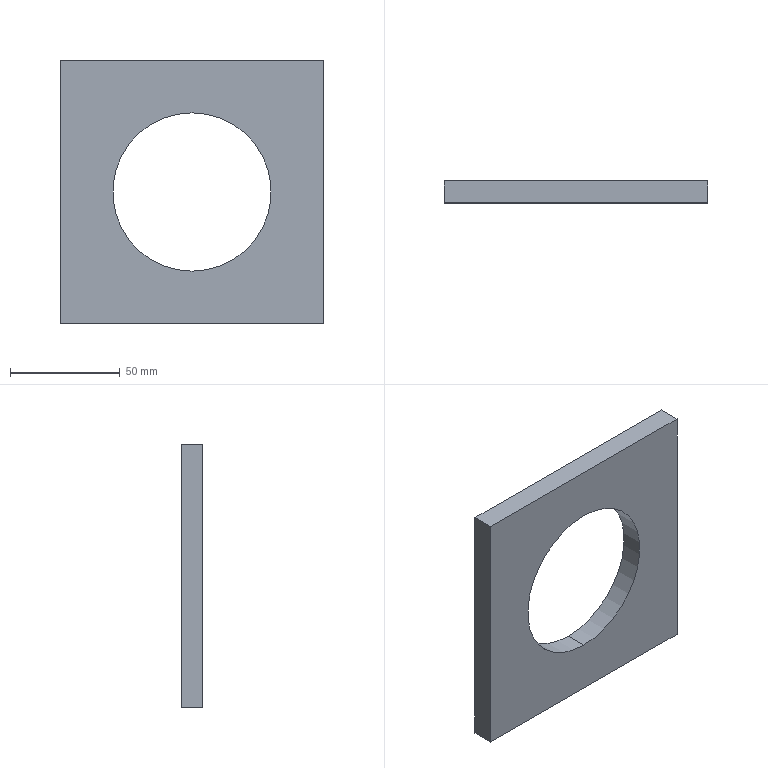Part | SolidWorks | features Extrusion 1 | 1 solid | 8 faces | box 120 x 10 x 120 mm | volume 103285 mm3 | plane 6 | cylinder 2 | commonest cylinder face diameters 72 x2
STEP:
#1=CARTESIAN_POINT('',(521.231,809.896,-476.693));
#2=VERTEX_POINT('',#1);
#3=CARTESIAN_POINT('',(521.231,809.896,-404.693));
#4=VERTEX_POINT('',#3);
#5=CARTESIAN_POINT('',(521.231,809.896,-440.693));
#6=DIRECTION('',(0.,1.,0.));
#7=DIRECTION('',(0.,0.,-1.));
#8=AXIS2_PLACEMENT_3D('',#5,#6,#7);
#9=CIRCLE('',#8,36.);
#10=EDGE_CURVE('',#2,#4,#9,.T.);
#11=ORIENTED_EDGE('',*,*,#10,.F.);
#12=CARTESIAN_POINT('',(521.231,819.896,-476.693));
#13=VERTEX_POINT('',#12);
#14=CARTESIAN_POINT('',(521.231,809.896,-476.693));
#15=DIRECTION('',(0.,1.,0.));
#16=VECTOR('',#15,1000.);
#17=LINE('',#14,#16);
#18=EDGE_CURVE('',#2,#13,#17,.T.);
#19=ORIENTED_EDGE('',*,*,#18,.T.);
#20=CARTESIAN_POINT('',(521.231,819.896,-404.693));
#21=VERTEX_POINT('',#20);
#22=CARTESIAN_POINT('',(521.231,819.896,-440.693));
#23=DIRECTION('',(0.,1.,0.));
#24=DIRECTION('',(0.,0.,-1.));
#25=AXIS2_PLACEMENT_3D('',#22,#23,#24);
#26=CIRCLE('',#25,36.);
#27=EDGE_CURVE('',#13,#21,#26,.T.);
#28=ORIENTED_EDGE('',*,*,#27,.T.);
#29=CARTESIAN_POINT('',(521.231,809.896,-404.693));
#30=DIRECTION('',(0.,1.,0.));
#31=VECTOR('',#30,1000.);
#32=LINE('',#29,#31);
#33=EDGE_CURVE('',#4,#21,#32,.T.);
#34=ORIENTED_EDGE('',*,*,#33,.F.);
#35=EDGE_LOOP('',(#11,#19,#28,#34));
#36=FACE_OUTER_BOUND('',#35,.T.);
#37=CARTESIAN_POINT('',(521.231,809.896,-440.693));
#38=DIRECTION('',(0.,1.,0.));
#39=DIRECTION('',(0.,0.,1.));
#40=AXIS2_PLACEMENT_3D('',#37,#38,#39);
#41=CYLINDRICAL_SURFACE('',#40,36.);
#42=ADVANCED_FACE('',(#36),#41,.F.);
#43=CARTESIAN_POINT('',(461.231,819.896,-380.693));
#44=VERTEX_POINT('',#43);
#45=CARTESIAN_POINT('',(581.231,819.896,-380.693));
#46=VERTEX_POINT('',#45);
#47=CARTESIAN_POINT('',(461.231,819.896,-380.693));
#48=DIRECTION('',(1.,0.,0.));
#49=VECTOR('',#48,1000.);
#50=LINE('',#47,#49);
#51=EDGE_CURVE('',#44,#46,#50,.T.);
#52=ORIENTED_EDGE('',*,*,#51,.F.);
#53=CARTESIAN_POINT('',(461.231,809.896,-380.693));
#54=VERTEX_POINT('',#53);
#55=CARTESIAN_POINT('',(461.231,809.896,-380.693));
#56=DIRECTION('',(0.,1.,0.));
#57=VECTOR('',#56,1000.);
#58=LINE('',#55,#57);
#59=EDGE_CURVE('',#54,#44,#58,.T.);
#60=ORIENTED_EDGE('',*,*,#59,.F.);
#61=CARTESIAN_POINT('',(581.231,809.896,-380.693));
#62=VERTEX_POINT('',#61);
#63=CARTESIAN_POINT('',(461.231,809.896,-380.693));
#64=DIRECTION('',(1.,0.,0.));
#65=VECTOR('',#64,1000.);
#66=LINE('',#63,#65);
#67=EDGE_CURVE('',#54,#62,#66,.T.);
#68=ORIENTED_EDGE('',*,*,#67,.T.);
#69=CARTESIAN_POINT('',(581.231,809.896,-380.693));
#70=DIRECTION('',(0.,1.,0.));
#71=VECTOR('',#70,1000.);
#72=LINE('',#69,#71);
#73=EDGE_CURVE('',#62,#46,#72,.T.);
#74=ORIENTED_EDGE('',*,*,#73,.T.);
#75=EDGE_LOOP('',(#52,#60,#68,#74));
#76=FACE_OUTER_BOUND('',#75,.T.);
#77=CARTESIAN_POINT('',(461.231,809.896,-380.693));
#78=DIRECTION('',(0.,0.,1.));
#79=DIRECTION('',(1.,0.,0.));
#80=AXIS2_PLACEMENT_3D('',#77,#78,#79);
#81=PLANE('',#80);
#82=ADVANCED_FACE('',(#76),#81,.T.);
#83=CARTESIAN_POINT('',(461.231,819.896,-500.693));
#84=VERTEX_POINT('',#83);
#85=CARTESIAN_POINT('',(461.231,819.896,-500.693));
#86=DIRECTION('',(0.,0.,1.));
#87=VECTOR('',#86,1000.);
#88=LINE('',#85,#87);
#89=EDGE_CURVE('',#84,#44,#88,.T.);
#90=ORIENTED_EDGE('',*,*,#89,.F.);
#91=CARTESIAN_POINT('',(461.231,809.896,-500.693));
#92=VERTEX_POINT('',#91);
#93=CARTESIAN_POINT('',(461.231,809.896,-500.693));
#94=DIRECTION('',(0.,1.,0.));
#95=VECTOR('',#94,1000.);
#96=LINE('',#93,#95);
#97=EDGE_CURVE('',#92,#84,#96,.T.);
#98=ORIENTED_EDGE('',*,*,#97,.F.);
#99=CARTESIAN_POINT('',(461.231,809.896,-500.693));
#100=DIRECTION('',(0.,0.,1.));
#101=VECTOR('',#100,1000.);
#102=LINE('',#99,#101);
#103=EDGE_CURVE('',#92,#54,#102,.T.);
#104=ORIENTED_EDGE('',*,*,#103,.T.);
#105=ORIENTED_EDGE('',*,*,#59,.T.);
#106=EDGE_LOOP('',(#90,#98,#104,#105));
#107=FACE_OUTER_BOUND('',#106,.T.);
#108=CARTESIAN_POINT('',(461.231,809.896,-500.693));
#109=DIRECTION('',(-1.,0.,0.));
#110=DIRECTION('',(0.,0.,1.));
#111=AXIS2_PLACEMENT_3D('',#108,#109,#110);
#112=PLANE('',#111);
#113=ADVANCED_FACE('',(#107),#112,.T.);
#114=CARTESIAN_POINT('',(581.231,819.896,-500.693));
#115=VERTEX_POINT('',#114);
#116=CARTESIAN_POINT('',(581.231,819.896,-500.693));
#117=DIRECTION('',(-1.,0.,0.));
#118=VECTOR('',#117,1000.);
#119=LINE('',#116,#118);
#120=EDGE_CURVE('',#115,#84,#119,.T.);
#121=ORIENTED_EDGE('',*,*,#120,.F.);
#122=CARTESIAN_POINT('',(581.231,809.896,-500.693));
#123=VERTEX_POINT('',#122);
#124=CARTESIAN_POINT('',(581.231,809.896,-500.693));
#125=DIRECTION('',(0.,1.,0.));
#126=VECTOR('',#125,1000.);
#127=LINE('',#124,#126);
#128=EDGE_CURVE('',#123,#115,#127,.T.);
#129=ORIENTED_EDGE('',*,*,#128,.F.);
#130=CARTESIAN_POINT('',(581.231,809.896,-500.693));
#131=DIRECTION('',(-1.,0.,0.));
#132=VECTOR('',#131,1000.);
#133=LINE('',#130,#132);
#134=EDGE_CURVE('',#123,#92,#133,.T.);
#135=ORIENTED_EDGE('',*,*,#134,.T.);
#136=ORIENTED_EDGE('',*,*,#97,.T.);
#137=EDGE_LOOP('',(#121,#129,#135,#136));
#138=FACE_OUTER_BOUND('',#137,.T.);
#139=CARTESIAN_POINT('',(581.231,809.896,-500.693));
#140=DIRECTION('',(0.,0.,-1.));
#141=DIRECTION('',(-1.,0.,0.));
#142=AXIS2_PLACEMENT_3D('',#139,#140,#141);
#143=PLANE('',#142);
#144=ADVANCED_FACE('',(#138),#143,.T.);
#145=CARTESIAN_POINT('',(581.231,819.896,-380.693));
#146=DIRECTION('',(0.,0.,-1.));
#147=VECTOR('',#146,1000.);
#148=LINE('',#145,#147);
#149=EDGE_CURVE('',#46,#115,#148,.T.);
#150=ORIENTED_EDGE('',*,*,#149,.F.);
#151=ORIENTED_EDGE('',*,*,#73,.F.);
#152=CARTESIAN_POINT('',(581.231,809.896,-380.693));
#153=DIRECTION('',(0.,0.,-1.));
#154=VECTOR('',#153,1000.);
#155=LINE('',#152,#154);
#156=EDGE_CURVE('',#62,#123,#155,.T.);
#157=ORIENTED_EDGE('',*,*,#156,.T.);
#158=ORIENTED_EDGE('',*,*,#128,.T.);
#159=EDGE_LOOP('',(#150,#151,#157,#158));
#160=FACE_OUTER_BOUND('',#159,.T.);
#161=CARTESIAN_POINT('',(581.231,809.896,-380.693));
#162=DIRECTION('',(1.,0.,0.));
#163=DIRECTION('',(0.,0.,-1.));
#164=AXIS2_PLACEMENT_3D('',#161,#162,#163);
#165=PLANE('',#164);
#166=ADVANCED_FACE('',(#160),#165,.T.);
#167=CARTESIAN_POINT('',(521.231,809.896,-440.693));
#168=DIRECTION('',(0.,1.,0.));
#169=DIRECTION('',(0.,0.,-1.));
#170=AXIS2_PLACEMENT_3D('',#167,#168,#169);
#171=CIRCLE('',#170,36.);
#172=EDGE_CURVE('',#4,#2,#171,.T.);
#173=ORIENTED_EDGE('',*,*,#172,.T.);
#174=ORIENTED_EDGE('',*,*,#10,.T.);
#175=EDGE_LOOP('',(#173,#174));
#176=FACE_BOUND('',#175,.T.);
#177=ORIENTED_EDGE('',*,*,#67,.F.);
#178=ORIENTED_EDGE('',*,*,#103,.F.);
#179=ORIENTED_EDGE('',*,*,#134,.F.);
#180=ORIENTED_EDGE('',*,*,#156,.F.);
#181=EDGE_LOOP('',(#177,#178,#179,#180));
#182=FACE_OUTER_BOUND('',#181,.T.);
#183=CARTESIAN_POINT('',(0.,809.896,0.));
#184=DIRECTION('',(0.,1.,0.));
#185=DIRECTION('',(0.,0.,1.));
#186=AXIS2_PLACEMENT_3D('',#183,#184,#185);
#187=PLANE('',#186);
#188=ADVANCED_FACE('',(#176,#182),#187,.F.);
#189=CARTESIAN_POINT('',(521.231,819.896,-440.693));
#190=DIRECTION('',(0.,1.,0.));
#191=DIRECTION('',(0.,0.,-1.));
#192=AXIS2_PLACEMENT_3D('',#189,#190,#191);
#193=CIRCLE('',#192,36.);
#194=EDGE_CURVE('',#21,#13,#193,.T.);
#195=ORIENTED_EDGE('',*,*,#194,.F.);
#196=ORIENTED_EDGE('',*,*,#27,.F.);
#197=EDGE_LOOP('',(#195,#196));
#198=FACE_BOUND('',#197,.T.);
#199=ORIENTED_EDGE('',*,*,#51,.T.);
#200=ORIENTED_EDGE('',*,*,#149,.T.);
#201=ORIENTED_EDGE('',*,*,#120,.T.);
#202=ORIENTED_EDGE('',*,*,#89,.T.);
#203=EDGE_LOOP('',(#199,#200,#201,#202));
#204=FACE_OUTER_BOUND('',#203,.T.);
#205=CARTESIAN_POINT('',(0.,819.896,0.));
#206=DIRECTION('',(0.,1.,0.));
#207=DIRECTION('',(0.,0.,1.));
#208=AXIS2_PLACEMENT_3D('',#205,#206,#207);
#209=PLANE('',#208);
#210=ADVANCED_FACE('',(#198,#204),#209,.T.);
#211=ORIENTED_EDGE('',*,*,#18,.F.);
#212=ORIENTED_EDGE('',*,*,#172,.F.);
#213=ORIENTED_EDGE('',*,*,#33,.T.);
#214=ORIENTED_EDGE('',*,*,#194,.T.);
#215=EDGE_LOOP('',(#211,#212,#213,#214));
#216=FACE_OUTER_BOUND('',#215,.T.);
#217=CARTESIAN_POINT('',(521.231,809.896,-440.693));
#218=DIRECTION('',(0.,1.,0.));
#219=DIRECTION('',(0.,0.,1.));
#220=AXIS2_PLACEMENT_3D('',#217,#218,#219);
#221=CYLINDRICAL_SURFACE('',#220,36.);
#222=ADVANCED_FACE('',(#216),#221,.F.);
#223=CLOSED_SHELL('',(#42,#82,#113,#144,#166,#188,#210,#222));
#224=MANIFOLD_SOLID_BREP('',#223);
#225=CARTESIAN_POINT('',(0.,0.,0.));
#226=DIRECTION('',(0.,0.,1.));
#227=DIRECTION('',(1.,0.,0.));
#228=AXIS2_PLACEMENT_3D('',#225,#226,#227);
#229=(LENGTH_UNIT()NAMED_UNIT(*)SI_UNIT(.MILLI.,.METRE.));
#230=UNCERTAINTY_MEASURE_WITH_UNIT(LENGTH_MEASURE(0.00001),#229,'','');
#231=(NAMED_UNIT(*)PLANE_ANGLE_UNIT()SI_UNIT($,.RADIAN.));
#232=(NAMED_UNIT(*)SI_UNIT($,.STERADIAN.)SOLID_ANGLE_UNIT());
#233=(GEOMETRIC_REPRESENTATION_CONTEXT(3)GLOBAL_UNCERTAINTY_ASSIGNED_CONTEXT((#230))GLOBAL_UNIT_ASSIGNED_CONTEXT((#229,#231,#232))REPRESENTATION_CONTEXT('',''));
#234=ADVANCED_BREP_SHAPE_REPRESENTATION('',(#224,#228),#233);